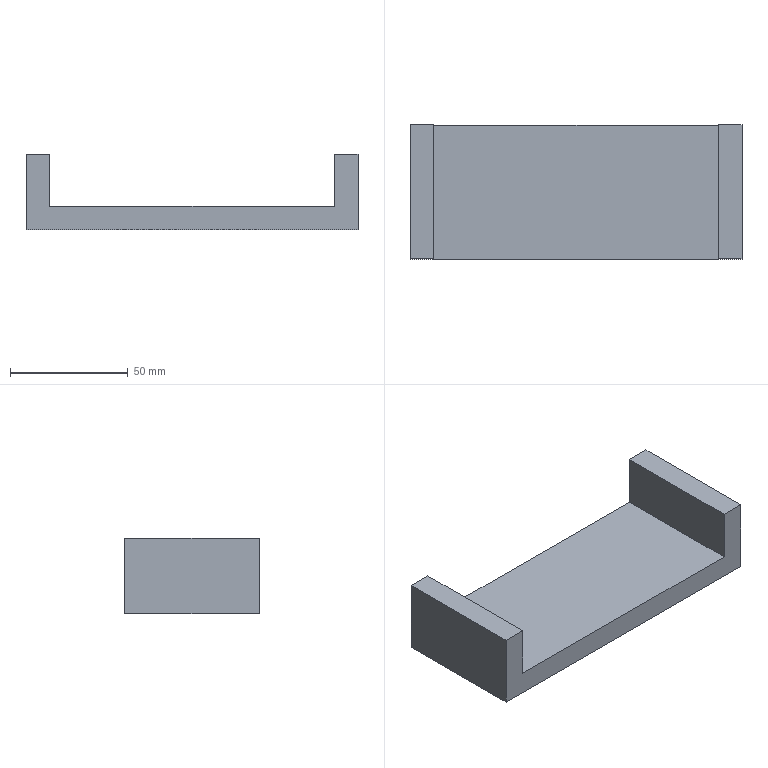Part | NX | features solid 2 | 1 solid | 10 faces | box 141.082 x 56.961 x 32.177 mm | volume 105625 mm3 | plane 10
STEP:
#1=CARTESIAN_POINT('',(8.041,151.934,-967.953));
#2=VERTEX_POINT('',#1);
#3=CARTESIAN_POINT('',(18.041,151.934,-967.953));
#4=VERTEX_POINT('',#3);
#5=CARTESIAN_POINT('',(-52.5,151.934,-967.953));
#6=DIRECTION('',(1.,0.,0.));
#7=VECTOR('',#6,1000.);
#8=LINE('',#5,#7);
#9=EDGE_CURVE('',#2,#4,#8,.T.);
#10=ORIENTED_EDGE('',*,*,#9,.F.);
#11=CARTESIAN_POINT('',(8.041,94.973,-967.953));
#12=VERTEX_POINT('',#11);
#13=CARTESIAN_POINT('',(8.041,123.454,-967.953));
#14=DIRECTION('',(0.,-1.,0.));
#15=VECTOR('',#14,1000.);
#16=LINE('',#13,#15);
#17=EDGE_CURVE('',#2,#12,#16,.T.);
#18=ORIENTED_EDGE('',*,*,#17,.T.);
#19=CARTESIAN_POINT('',(18.041,94.973,-967.953));
#20=VERTEX_POINT('',#19);
#21=CARTESIAN_POINT('',(-52.5,94.973,-967.953));
#22=DIRECTION('',(-1.,0.,0.));
#23=VECTOR('',#22,1000.);
#24=LINE('',#21,#23);
#25=EDGE_CURVE('',#20,#12,#24,.T.);
#26=ORIENTED_EDGE('',*,*,#25,.F.);
#27=CARTESIAN_POINT('',(18.041,123.454,-967.953));
#28=DIRECTION('',(0.,-1.,0.));
#29=VECTOR('',#28,1000.);
#30=LINE('',#27,#29);
#31=EDGE_CURVE('',#4,#20,#30,.T.);
#32=ORIENTED_EDGE('',*,*,#31,.F.);
#33=EDGE_LOOP('',(#10,#18,#26,#32));
#34=FACE_BOUND('',#33,.T.);
#35=CARTESIAN_POINT('',(-52.5,123.454,-967.953));
#36=DIRECTION('',(0.,0.,1.));
#37=DIRECTION('',(1.,0.,0.));
#38=AXIS2_PLACEMENT_3D('',#35,#36,#37);
#39=PLANE('',#38);
#40=ADVANCED_FACE('',(#34),#39,.T.);
#41=CARTESIAN_POINT('',(-113.041,94.973,-967.953));
#42=VERTEX_POINT('',#41);
#43=CARTESIAN_POINT('',(-123.041,94.973,-967.953));
#44=VERTEX_POINT('',#43);
#45=CARTESIAN_POINT('',(-52.5,94.973,-967.953));
#46=DIRECTION('',(-1.,0.,0.));
#47=VECTOR('',#46,1000.);
#48=LINE('',#45,#47);
#49=EDGE_CURVE('',#42,#44,#48,.T.);
#50=ORIENTED_EDGE('',*,*,#49,.F.);
#51=CARTESIAN_POINT('',(-113.041,151.934,-967.953));
#52=VERTEX_POINT('',#51);
#53=CARTESIAN_POINT('',(-113.041,123.454,-967.953));
#54=DIRECTION('',(0.,1.,0.));
#55=VECTOR('',#54,1000.);
#56=LINE('',#53,#55);
#57=EDGE_CURVE('',#42,#52,#56,.T.);
#58=ORIENTED_EDGE('',*,*,#57,.T.);
#59=CARTESIAN_POINT('',(-123.041,151.934,-967.953));
#60=VERTEX_POINT('',#59);
#61=CARTESIAN_POINT('',(-52.5,151.934,-967.953));
#62=DIRECTION('',(1.,0.,0.));
#63=VECTOR('',#62,1000.);
#64=LINE('',#61,#63);
#65=EDGE_CURVE('',#60,#52,#64,.T.);
#66=ORIENTED_EDGE('',*,*,#65,.F.);
#67=CARTESIAN_POINT('',(-123.041,123.454,-967.953));
#68=DIRECTION('',(0.,1.,0.));
#69=VECTOR('',#68,1000.);
#70=LINE('',#67,#69);
#71=EDGE_CURVE('',#44,#60,#70,.T.);
#72=ORIENTED_EDGE('',*,*,#71,.F.);
#73=EDGE_LOOP('',(#50,#58,#66,#72));
#74=FACE_BOUND('',#73,.T.);
#75=CARTESIAN_POINT('',(-52.5,123.454,-967.953));
#76=DIRECTION('',(0.,0.,1.));
#77=DIRECTION('',(1.,0.,0.));
#78=AXIS2_PLACEMENT_3D('',#75,#76,#77);
#79=PLANE('',#78);
#80=ADVANCED_FACE('',(#74),#79,.T.);
#81=CARTESIAN_POINT('',(8.041,94.973,-990.129));
#82=VERTEX_POINT('',#81);
#83=CARTESIAN_POINT('',(8.041,94.973,-985.349));
#84=DIRECTION('',(0.,0.,1.));
#85=VECTOR('',#84,1000.);
#86=LINE('',#83,#85);
#87=EDGE_CURVE('',#82,#12,#86,.T.);
#88=ORIENTED_EDGE('',*,*,#87,.F.);
#89=CARTESIAN_POINT('',(-113.041,94.973,-990.129));
#90=VERTEX_POINT('',#89);
#91=CARTESIAN_POINT('',(-52.5,94.973,-990.129));
#92=DIRECTION('',(-1.,0.,0.));
#93=VECTOR('',#92,1000.);
#94=LINE('',#91,#93);
#95=EDGE_CURVE('',#90,#82,#94,.F.);
#96=ORIENTED_EDGE('',*,*,#95,.F.);
#97=CARTESIAN_POINT('',(-113.041,94.973,-985.349));
#98=DIRECTION('',(0.,0.,1.));
#99=VECTOR('',#98,1000.);
#100=LINE('',#97,#99);
#101=EDGE_CURVE('',#90,#42,#100,.T.);
#102=ORIENTED_EDGE('',*,*,#101,.T.);
#103=ORIENTED_EDGE('',*,*,#49,.T.);
#104=CARTESIAN_POINT('',(-123.041,94.973,-1000.129));
#105=VERTEX_POINT('',#104);
#106=CARTESIAN_POINT('',(-123.041,94.973,-985.349));
#107=DIRECTION('',(0.,0.,1.));
#108=VECTOR('',#107,1000.);
#109=LINE('',#106,#108);
#110=EDGE_CURVE('',#105,#44,#109,.T.);
#111=ORIENTED_EDGE('',*,*,#110,.F.);
#112=CARTESIAN_POINT('',(18.041,94.973,-1000.129));
#113=VERTEX_POINT('',#112);
#114=CARTESIAN_POINT('',(-52.5,94.973,-1000.129));
#115=DIRECTION('',(-1.,0.,0.));
#116=VECTOR('',#115,1000.);
#117=LINE('',#114,#116);
#118=EDGE_CURVE('',#105,#113,#117,.F.);
#119=ORIENTED_EDGE('',*,*,#118,.T.);
#120=CARTESIAN_POINT('',(18.041,94.973,-985.349));
#121=DIRECTION('',(0.,0.,1.));
#122=VECTOR('',#121,1000.);
#123=LINE('',#120,#122);
#124=EDGE_CURVE('',#113,#20,#123,.T.);
#125=ORIENTED_EDGE('',*,*,#124,.T.);
#126=ORIENTED_EDGE('',*,*,#25,.T.);
#127=EDGE_LOOP('',(#88,#96,#102,#103,#111,#119,#125,#126));
#128=FACE_BOUND('',#127,.T.);
#129=CARTESIAN_POINT('',(-52.5,94.973,-985.349));
#130=DIRECTION('',(0.,-1.,0.));
#131=DIRECTION('',(0.,0.,-1.));
#132=AXIS2_PLACEMENT_3D('',#129,#130,#131);
#133=PLANE('',#132);
#134=ADVANCED_FACE('',(#128),#133,.T.);
#135=ORIENTED_EDGE('',*,*,#110,.T.);
#136=ORIENTED_EDGE('',*,*,#71,.T.);
#137=CARTESIAN_POINT('',(-123.041,151.934,-1000.129));
#138=VERTEX_POINT('',#137);
#139=CARTESIAN_POINT('',(-123.041,151.934,-985.349));
#140=DIRECTION('',(0.,0.,1.));
#141=VECTOR('',#140,1000.);
#142=LINE('',#139,#141);
#143=EDGE_CURVE('',#138,#60,#142,.T.);
#144=ORIENTED_EDGE('',*,*,#143,.F.);
#145=CARTESIAN_POINT('',(-123.041,123.454,-1000.129));
#146=DIRECTION('',(0.,1.,0.));
#147=VECTOR('',#146,1000.);
#148=LINE('',#145,#147);
#149=EDGE_CURVE('',#138,#105,#148,.F.);
#150=ORIENTED_EDGE('',*,*,#149,.T.);
#151=EDGE_LOOP('',(#135,#136,#144,#150));
#152=FACE_BOUND('',#151,.T.);
#153=CARTESIAN_POINT('',(-123.041,123.454,-985.349));
#154=DIRECTION('',(-1.,0.,0.));
#155=DIRECTION('',(0.,0.,1.));
#156=AXIS2_PLACEMENT_3D('',#153,#154,#155);
#157=PLANE('',#156);
#158=ADVANCED_FACE('',(#152),#157,.T.);
#159=CARTESIAN_POINT('',(-113.041,151.934,-990.129));
#160=VERTEX_POINT('',#159);
#161=CARTESIAN_POINT('',(-113.041,151.934,-985.349));
#162=DIRECTION('',(0.,0.,1.));
#163=VECTOR('',#162,1000.);
#164=LINE('',#161,#163);
#165=EDGE_CURVE('',#160,#52,#164,.T.);
#166=ORIENTED_EDGE('',*,*,#165,.F.);
#167=CARTESIAN_POINT('',(8.041,151.934,-990.129));
#168=VERTEX_POINT('',#167);
#169=CARTESIAN_POINT('',(-52.5,151.934,-990.129));
#170=DIRECTION('',(1.,0.,0.));
#171=VECTOR('',#170,1000.);
#172=LINE('',#169,#171);
#173=EDGE_CURVE('',#168,#160,#172,.F.);
#174=ORIENTED_EDGE('',*,*,#173,.F.);
#175=CARTESIAN_POINT('',(8.041,151.934,-985.349));
#176=DIRECTION('',(0.,0.,1.));
#177=VECTOR('',#176,1000.);
#178=LINE('',#175,#177);
#179=EDGE_CURVE('',#168,#2,#178,.T.);
#180=ORIENTED_EDGE('',*,*,#179,.T.);
#181=ORIENTED_EDGE('',*,*,#9,.T.);
#182=CARTESIAN_POINT('',(18.041,151.934,-1000.129));
#183=VERTEX_POINT('',#182);
#184=CARTESIAN_POINT('',(18.041,151.934,-985.349));
#185=DIRECTION('',(0.,0.,1.));
#186=VECTOR('',#185,1000.);
#187=LINE('',#184,#186);
#188=EDGE_CURVE('',#183,#4,#187,.T.);
#189=ORIENTED_EDGE('',*,*,#188,.F.);
#190=CARTESIAN_POINT('',(-52.5,151.934,-1000.129));
#191=DIRECTION('',(1.,0.,0.));
#192=VECTOR('',#191,1000.);
#193=LINE('',#190,#192);
#194=EDGE_CURVE('',#183,#138,#193,.F.);
#195=ORIENTED_EDGE('',*,*,#194,.T.);
#196=ORIENTED_EDGE('',*,*,#143,.T.);
#197=ORIENTED_EDGE('',*,*,#65,.T.);
#198=EDGE_LOOP('',(#166,#174,#180,#181,#189,#195,#196,#197));
#199=FACE_BOUND('',#198,.T.);
#200=CARTESIAN_POINT('',(-52.5,151.934,-985.349));
#201=DIRECTION('',(0.,1.,0.));
#202=DIRECTION('',(0.,0.,1.));
#203=AXIS2_PLACEMENT_3D('',#200,#201,#202);
#204=PLANE('',#203);
#205=ADVANCED_FACE('',(#199),#204,.T.);
#206=CARTESIAN_POINT('',(18.041,123.454,-1000.129));
#207=DIRECTION('',(0.,-1.,0.));
#208=VECTOR('',#207,1000.);
#209=LINE('',#206,#208);
#210=EDGE_CURVE('',#113,#183,#209,.F.);
#211=ORIENTED_EDGE('',*,*,#210,.F.);
#212=ORIENTED_EDGE('',*,*,#118,.F.);
#213=ORIENTED_EDGE('',*,*,#149,.F.);
#214=ORIENTED_EDGE('',*,*,#194,.F.);
#215=EDGE_LOOP('',(#211,#212,#213,#214));
#216=FACE_BOUND('',#215,.T.);
#217=CARTESIAN_POINT('',(43.3,-194.,-1000.129));
#218=DIRECTION('',(0.,0.,1.));
#219=DIRECTION('',(0.,1.,0.));
#220=AXIS2_PLACEMENT_3D('',#217,#218,#219);
#221=PLANE('',#220);
#222=ADVANCED_FACE('',(#216),#221,.F.);
#223=ORIENTED_EDGE('',*,*,#210,.T.);
#224=ORIENTED_EDGE('',*,*,#188,.T.);
#225=ORIENTED_EDGE('',*,*,#31,.T.);
#226=ORIENTED_EDGE('',*,*,#124,.F.);
#227=EDGE_LOOP('',(#223,#224,#225,#226));
#228=FACE_BOUND('',#227,.T.);
#229=CARTESIAN_POINT('',(18.041,123.454,-985.349));
#230=DIRECTION('',(1.,0.,0.));
#231=DIRECTION('',(0.,0.,-1.));
#232=AXIS2_PLACEMENT_3D('',#229,#230,#231);
#233=PLANE('',#232);
#234=ADVANCED_FACE('',(#228),#233,.T.);
#235=ORIENTED_EDGE('',*,*,#101,.F.);
#236=CARTESIAN_POINT('',(-113.041,123.454,-990.129));
#237=DIRECTION('',(0.,1.,0.));
#238=VECTOR('',#237,1000.);
#239=LINE('',#236,#238);
#240=EDGE_CURVE('',#160,#90,#239,.F.);
#241=ORIENTED_EDGE('',*,*,#240,.F.);
#242=ORIENTED_EDGE('',*,*,#165,.T.);
#243=ORIENTED_EDGE('',*,*,#57,.F.);
#244=EDGE_LOOP('',(#235,#241,#242,#243));
#245=FACE_BOUND('',#244,.T.);
#246=CARTESIAN_POINT('',(-113.041,123.454,-985.349));
#247=DIRECTION('',(-1.,0.,0.));
#248=DIRECTION('',(0.,0.,1.));
#249=AXIS2_PLACEMENT_3D('',#246,#247,#248);
#250=PLANE('',#249);
#251=ADVANCED_FACE('',(#245),#250,.F.);
#252=CARTESIAN_POINT('',(8.041,123.454,-990.129));
#253=DIRECTION('',(0.,-1.,0.));
#254=VECTOR('',#253,1000.);
#255=LINE('',#252,#254);
#256=EDGE_CURVE('',#82,#168,#255,.F.);
#257=ORIENTED_EDGE('',*,*,#256,.T.);
#258=ORIENTED_EDGE('',*,*,#173,.T.);
#259=ORIENTED_EDGE('',*,*,#240,.T.);
#260=ORIENTED_EDGE('',*,*,#95,.T.);
#261=EDGE_LOOP('',(#257,#258,#259,#260));
#262=FACE_BOUND('',#261,.T.);
#263=CARTESIAN_POINT('',(43.3,-194.,-990.129));
#264=DIRECTION('',(0.,0.,1.));
#265=DIRECTION('',(0.,1.,0.));
#266=AXIS2_PLACEMENT_3D('',#263,#264,#265);
#267=PLANE('',#266);
#268=ADVANCED_FACE('',(#262),#267,.T.);
#269=ORIENTED_EDGE('',*,*,#256,.F.);
#270=ORIENTED_EDGE('',*,*,#87,.T.);
#271=ORIENTED_EDGE('',*,*,#17,.F.);
#272=ORIENTED_EDGE('',*,*,#179,.F.);
#273=EDGE_LOOP('',(#269,#270,#271,#272));
#274=FACE_BOUND('',#273,.T.);
#275=CARTESIAN_POINT('',(8.041,123.454,-985.349));
#276=DIRECTION('',(1.,0.,0.));
#277=DIRECTION('',(0.,0.,-1.));
#278=AXIS2_PLACEMENT_3D('',#275,#276,#277);
#279=PLANE('',#278);
#280=ADVANCED_FACE('',(#274),#279,.F.);
#281=CLOSED_SHELL('',(#40,#80,#134,#158,#205,#222,#234,#251,#268,#280));
#282=MANIFOLD_SOLID_BREP('',#281);
#283=(LENGTH_UNIT()NAMED_UNIT(*)SI_UNIT(.MILLI.,.METRE.));
#284=UNCERTAINTY_MEASURE_WITH_UNIT(LENGTH_MEASURE(0.00001),#283,'','');
#285=(NAMED_UNIT(*)PLANE_ANGLE_UNIT()SI_UNIT($,.RADIAN.));
#286=(NAMED_UNIT(*)SI_UNIT($,.STERADIAN.)SOLID_ANGLE_UNIT());
#287=(GEOMETRIC_REPRESENTATION_CONTEXT(3)GLOBAL_UNCERTAINTY_ASSIGNED_CONTEXT((#284))GLOBAL_UNIT_ASSIGNED_CONTEXT((#283,#285,#286))REPRESENTATION_CONTEXT('',''));
#288=ADVANCED_BREP_SHAPE_REPRESENTATION('',(#282),#287);